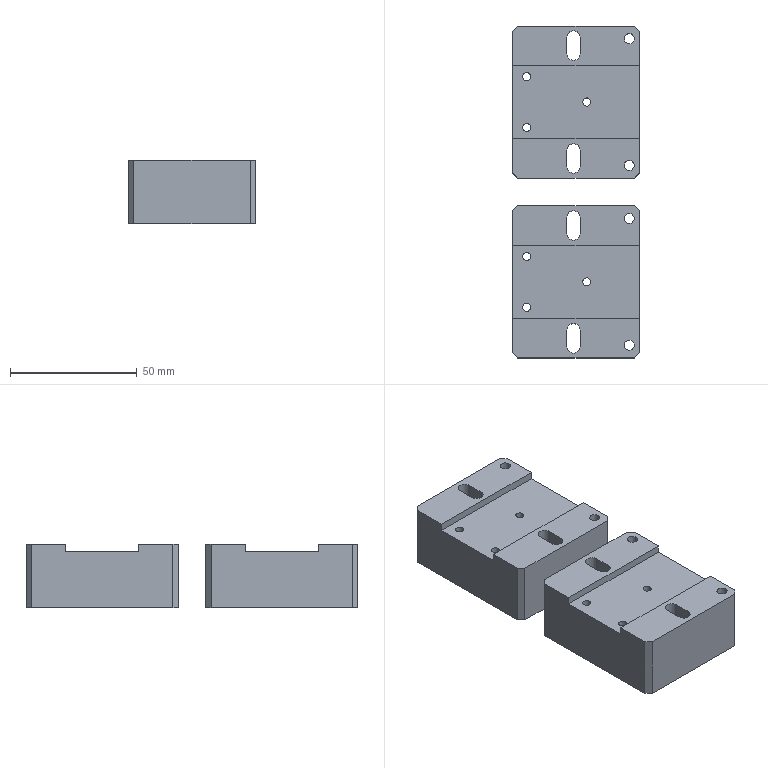CAM job | NX | 3-axis milling, drilling | part box 50 x 131 x 25 mm | stock box 55 x 135 x 30 mm
Tools:
number,name,description,diameter,corner_radius,flute_length,length,flutes
4,D4,平底铣刀-粗,4.0,0.0,25.0,75.0,2
9,D10,平底铣刀-粗,10.0,0.0,35.0,75.0,2
11,D4-J,平底铣刀-精,4.0,0.0,50.0,75.0,2
10,D10-J,平底铣刀-精,10.0,0.0,35.0,75.0,2
1,D80R0.8飞刀,圆鼻刀-粗,80.0,0.8,50.0,75.0,2
2,D6倒角刀,倒角刀,6.0,0.0,3.0,25.0,2
19,D4铰刀,Drilling Tool,4.0,0.0,75.0,100.0,6
18,ZT3.9,Drilling Tool,3.9,0.0,35.0,50.0,2
17,ZT3.2,Drilling Tool,3.2,0.0,35.0,50.0,2
Operations:
program,operation,operation_type,tool,method,geometry_group,spindle_rpm,surface_speed,feed_per_tooth,feed_cut,feed_plunge,cut_length_mm,path_length_mm,cut_time_min,machine_time_min
B,动态开粗D10_COPY,CavityMilling,D10,动态开粗-切深K-步距K,W-B,8000.0,251.32,0.25,4000.0,100.0,12459.086,12494.886,3.115,3.118
B,底壁铣分层开粗-中_COPY,VolumeBased25DMillingOperation,D10,分层开粗-切深K-步距G,W-B,8000.0,251.32,0.25,4000.0,100.0,2748.702,2862.888,0.6872,0.6986
B,C0.3封闭铣廓倒角6X45L_COPY_1,PlanarMilling,D6倒角刀,爬面_倒角-切深0-步距G,W-B,7000.0,131.0,0.1071,1500.0,100.0,583.517,919.168,0.389,0.4226
B,钻倒角_2,Operation,D6倒角刀,METHOD,W-B,8000.0,150.796,0.0625,1000.0,0.0,29.4,263.131,0.0294,0.0528
B,钻倒角_3,Operation,D6倒角刀,METHOD,W-B,8000.0,150.796,0.0625,1000.0,0.0,21.2,212.793,0.0212,0.0404
B,平面去毛刺6X45L_COPY,SurfaceContour,D6倒角刀,爬面_倒角-切深0-步距G,W-B,6500.0,122.519,0.1154,1500.0,100.0,862.347,1976.861,0.5749,0.6863
B,底壁铣飞面精光_COPY,VolumeBased25DMillingOperation,D10-J,侧刃精光-切深K-步距G,W-B,8000.0,251.32,0.0625,1000.0,100.0,1052.833,1088.833,1.053,1.056
B,底壁铣精光底面-中_COPY,VolumeBased25DMillingOperation,D10-J,精光步距切深关,W-B,8000.0,251.32,0.0625,1000.0,100.0,656.64,828.48,0.6566,0.6738
B,底壁铣精光侧面-中-选底面_COPY,VolumeBased25DMillingOperation,D10-J,侧刃精光-切深K-步距G,W-B,8000.0,251.32,0.0625,1000.0,100.0,272.772,431.038,0.2728,0.2886
A,C0.3封闭铣廓倒角6X45L_COPY,PlanarMilling,D6倒角刀,爬面_倒角-切深0-步距G,W-A,7000.0,131.0,0.1071,1500.0,100.0,465.684,608.729,0.3105,0.3248
A,顶面,FaceMilling,D80R0.8飞刀,侧刃精光-切深K-步距G,W-A,5000.0,1256.637,0.1,1000.0,100.0,225.0,261.0,0.225,0.2286
A,外形粗_2,VolumeBased25DMillingOperation,D10,METHOD,W-A,8000.0,251.327,0.3125,5000.0,80.0,16823.422,17021.522,3.365,3.385
A,打点-深0.8,Operation,D6倒角刀,NONE,W-A,8000.0,150.796,0.0312,500.0,90.0,32.4,626.873,0.0648,0.1242
A,沉头孔-钻孔0段,Operation,ZT3.2,NONE,W-A,2800.0,28.149,0.0357,200.0,90.0,155.543,498.63,0.7777,0.812
A,通孔-精孔4.0预钻,Operation,ZT3.9,NONE,W-A,3000.0,36.757,0.0417,250.0,90.0,361.51,1264.617,1.446,1.536
A,通腰槽粗_1,VolumeBased25DMillingOperation,D4,METHOD,W-A,6000.0,75.398,0.1667,2000.0,100.0,6808.438,7178.488,3.404,3.441
A,铣孔开粗D4_1,CylinderMilling,D4,NONE,W-A,8000.0,100.531,0.075,1200.0,100.0,900.317,1336.206,0.7503,0.7939
A,铣孔精光D4_1,CylinderMilling,D4-J,精光步距切深关,W-A,8000.0,100.531,0.0312,500.0,100.0,128.189,564.078,0.2564,0.3
A,腰槽精_1,VolumeBased25DMillingOperation,D4-J,METHOD,W-A,6000.0,113.0,0.0417,500.0,100.0,455.065,1139.527,0.9101,0.9786
A,仅选体,SurfaceContour,D6倒角刀,METHOD,W-A,8000.0,150.796,0.1875,3000.0,100.0,586.09,1014.109,0.1954,0.2382
A,钻倒角_1,Operation,D6倒角刀,METHOD,W-A,8000.0,150.796,0.0312,500.0,0.0,21.2,212.793,0.0424,0.0616
A,铣倒角_1,PlanarMilling,D6倒角刀,NONE,W-A,8000.0,150.796,0.0312,500.0,100.0,166.108,528.633,0.3322,0.3685
A,铰孔,Operation,D4铰刀,METHOD,W-A,500.0,6.283,0.0167,50.0,0.0,108.0,380.044,2.16,2.187
A,外形半精_2,VolumeBased25DMillingOperation,D10-J,METHOD,W-A,8000.0,251.327,0.0625,1000.0,100.0,1017.297,1422.063,1.017,1.058